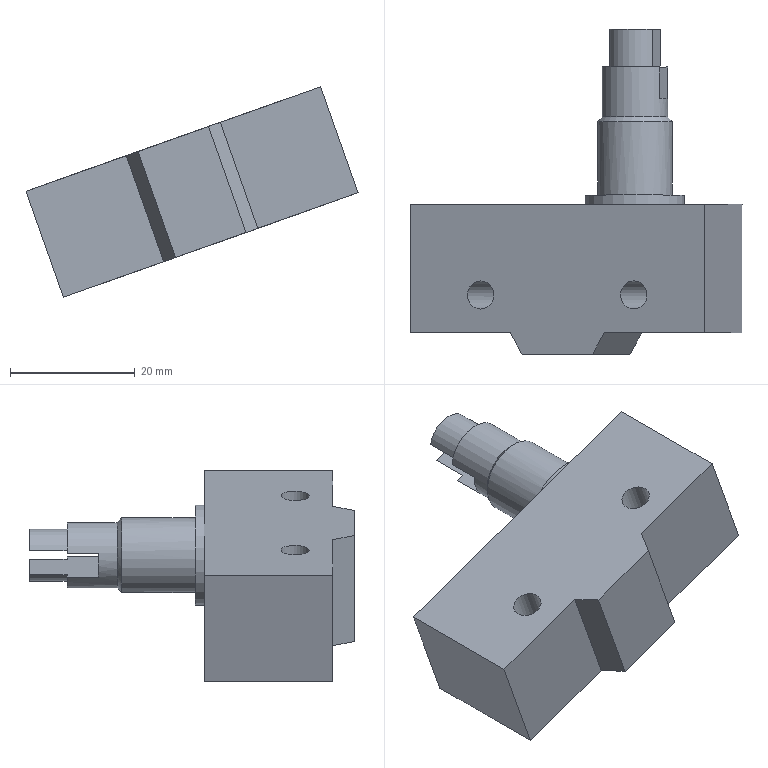Part | STEP file | ELECTRICAL-MICRO-SWITCH3_id10_x_t | 1 solid | 26 faces | box 53.141 x 52 x 33.658 mm | volume 21085 mm3 | plane 18 | cylinder 7 | cone 1 | commonest cylinder face diameters 4.5 x2 8.3 x2 10.5 x1 12 x1 16 x1
STEP:
#1=CARTESIAN_POINT('',(63.608,-176.5,-30.287));
#2=VERTEX_POINT('',#1);
#3=CARTESIAN_POINT('',(56.753,-176.5,-32.715));
#4=VERTEX_POINT('',#3);
#5=CARTESIAN_POINT('',(60.848,-176.5,-33.386));
#6=DIRECTION('',(0.,-1.,0.));
#7=DIRECTION('',(-0.9426,0.,-0.3338));
#8=AXIS2_PLACEMENT_3D('',#5,#6,#7);
#9=CIRCLE('',#8,4.15);
#10=EDGE_CURVE('',#2,#4,#9,.T.);
#11=ORIENTED_EDGE('',*,*,#10,.F.);
#12=CARTESIAN_POINT('',(63.608,-176.5,-30.287));
#13=DIRECTION('',(-0.9426,0.,-0.3338));
#14=VECTOR('',#13,1.);
#15=LINE('',#12,#14);
#16=EDGE_CURVE('',#2,#4,#15,.T.);
#17=ORIENTED_EDGE('',*,*,#16,.T.);
#18=EDGE_LOOP('',(#11,#17));
#19=FACE_OUTER_BOUND('',#18,.T.);
#20=CARTESIAN_POINT('',(60.848,-176.5,-33.386));
#21=DIRECTION('',(0.,1.,0.));
#22=DIRECTION('',(-0.9426,0.,-0.3338));
#23=AXIS2_PLACEMENT_3D('',#20,#21,#22);
#24=PLANE('',#23);
#25=ADVANCED_FACE('',(#19),#24,.T.);
#26=CARTESIAN_POINT('',(56.753,-182.5,-32.715));
#27=VERTEX_POINT('',#26);
#28=CARTESIAN_POINT('',(56.753,-176.5,-32.715));
#29=DIRECTION('',(0.,-1.,0.));
#30=VECTOR('',#29,1.);
#31=LINE('',#28,#30);
#32=EDGE_CURVE('',#4,#27,#31,.T.);
#33=ORIENTED_EDGE('',*,*,#32,.T.);
#34=CARTESIAN_POINT('',(63.608,-182.5,-30.287));
#35=VERTEX_POINT('',#34);
#36=CARTESIAN_POINT('',(60.848,-182.5,-33.386));
#37=DIRECTION('',(0.,-1.,0.));
#38=DIRECTION('',(-0.9426,0.,-0.3338));
#39=AXIS2_PLACEMENT_3D('',#36,#37,#38);
#40=CIRCLE('',#39,4.15);
#41=EDGE_CURVE('',#35,#27,#40,.T.);
#42=ORIENTED_EDGE('',*,*,#41,.F.);
#43=CARTESIAN_POINT('',(63.608,-182.5,-30.287));
#44=DIRECTION('',(0.,1.,0.));
#45=VECTOR('',#44,1.);
#46=LINE('',#43,#45);
#47=EDGE_CURVE('',#35,#2,#46,.T.);
#48=ORIENTED_EDGE('',*,*,#47,.T.);
#49=ORIENTED_EDGE('',*,*,#10,.T.);
#50=EDGE_LOOP('',(#33,#42,#48,#49));
#51=FACE_OUTER_BOUND('',#50,.T.);
#52=CARTESIAN_POINT('',(60.848,-204.325,-33.386));
#53=DIRECTION('',(0.,1.,0.));
#54=DIRECTION('',(-0.9426,0.,-0.3338));
#55=AXIS2_PLACEMENT_3D('',#52,#53,#54);
#56=CYLINDRICAL_SURFACE('',#55,4.15);
#57=ADVANCED_FACE('',(#51),#56,.T.);
#58=CARTESIAN_POINT('',(58.088,-176.5,-36.485));
#59=VERTEX_POINT('',#58);
#60=CARTESIAN_POINT('',(64.943,-176.5,-34.057));
#61=VERTEX_POINT('',#60);
#62=CARTESIAN_POINT('',(60.848,-176.5,-33.386));
#63=DIRECTION('',(0.,-1.,0.));
#64=DIRECTION('',(-0.9426,0.,-0.3338));
#65=AXIS2_PLACEMENT_3D('',#62,#63,#64);
#66=CIRCLE('',#65,4.15);
#67=EDGE_CURVE('',#59,#61,#66,.T.);
#68=ORIENTED_EDGE('',*,*,#67,.F.);
#69=CARTESIAN_POINT('',(58.088,-176.5,-36.485));
#70=DIRECTION('',(0.9426,0.,0.3338));
#71=VECTOR('',#70,1.);
#72=LINE('',#69,#71);
#73=EDGE_CURVE('',#59,#61,#72,.T.);
#74=ORIENTED_EDGE('',*,*,#73,.T.);
#75=EDGE_LOOP('',(#68,#74));
#76=FACE_OUTER_BOUND('',#75,.T.);
#77=CARTESIAN_POINT('',(60.848,-176.5,-33.386));
#78=DIRECTION('',(0.,1.,0.));
#79=DIRECTION('',(-0.9426,0.,-0.3338));
#80=AXIS2_PLACEMENT_3D('',#77,#78,#79);
#81=PLANE('',#80);
#82=ADVANCED_FACE('',(#76),#81,.T.);
#83=CARTESIAN_POINT('',(58.088,-182.5,-36.485));
#84=VERTEX_POINT('',#83);
#85=CARTESIAN_POINT('',(58.088,-182.5,-36.485));
#86=DIRECTION('',(0.,1.,0.));
#87=VECTOR('',#86,1.);
#88=LINE('',#85,#87);
#89=EDGE_CURVE('',#84,#59,#88,.T.);
#90=ORIENTED_EDGE('',*,*,#89,.T.);
#91=ORIENTED_EDGE('',*,*,#67,.T.);
#92=CARTESIAN_POINT('',(64.943,-182.5,-34.057));
#93=VERTEX_POINT('',#92);
#94=CARTESIAN_POINT('',(64.943,-176.5,-34.057));
#95=DIRECTION('',(0.,-1.,0.));
#96=VECTOR('',#95,1.);
#97=LINE('',#94,#96);
#98=EDGE_CURVE('',#61,#93,#97,.T.);
#99=ORIENTED_EDGE('',*,*,#98,.T.);
#100=CARTESIAN_POINT('',(60.848,-182.5,-33.386));
#101=DIRECTION('',(0.,-1.,0.));
#102=DIRECTION('',(-0.9426,0.,-0.3338));
#103=AXIS2_PLACEMENT_3D('',#100,#101,#102);
#104=CIRCLE('',#103,4.15);
#105=EDGE_CURVE('',#84,#93,#104,.T.);
#106=ORIENTED_EDGE('',*,*,#105,.F.);
#107=EDGE_LOOP('',(#90,#91,#99,#106));
#108=FACE_OUTER_BOUND('',#107,.T.);
#109=CARTESIAN_POINT('',(60.848,-204.325,-33.386));
#110=DIRECTION('',(0.,1.,0.));
#111=DIRECTION('',(-0.9426,0.,-0.3338));
#112=AXIS2_PLACEMENT_3D('',#109,#110,#111);
#113=CYLINDRICAL_SURFACE('',#112,4.15);
#114=ADVANCED_FACE('',(#108),#113,.T.);
#115=CARTESIAN_POINT('',(55.605,-187.5,-33.121));
#116=VERTEX_POINT('',#115);
#117=CARTESIAN_POINT('',(56.94,-187.5,-36.892));
#118=VERTEX_POINT('',#117);
#119=CARTESIAN_POINT('',(60.848,-187.5,-33.386));
#120=DIRECTION('',(0.,-1.,0.));
#121=DIRECTION('',(-0.9426,0.,-0.3338));
#122=AXIS2_PLACEMENT_3D('',#119,#120,#121);
#123=CIRCLE('',#122,5.25);
#124=EDGE_CURVE('',#116,#118,#123,.T.);
#125=ORIENTED_EDGE('',*,*,#124,.F.);
#126=CARTESIAN_POINT('',(64.756,-187.5,-29.88));
#127=VERTEX_POINT('',#126);
#128=CARTESIAN_POINT('',(55.605,-187.5,-33.121));
#129=DIRECTION('',(0.9426,0.,0.3338));
#130=VECTOR('',#129,1.);
#131=LINE('',#128,#130);
#132=EDGE_CURVE('',#116,#127,#131,.T.);
#133=ORIENTED_EDGE('',*,*,#132,.T.);
#134=CARTESIAN_POINT('',(66.091,-187.5,-33.651));
#135=VERTEX_POINT('',#134);
#136=CARTESIAN_POINT('',(60.848,-187.5,-33.386));
#137=DIRECTION('',(0.,-1.,0.));
#138=DIRECTION('',(-0.9426,0.,-0.3338));
#139=AXIS2_PLACEMENT_3D('',#136,#137,#138);
#140=CIRCLE('',#139,5.25);
#141=EDGE_CURVE('',#135,#127,#140,.T.);
#142=ORIENTED_EDGE('',*,*,#141,.F.);
#143=CARTESIAN_POINT('',(66.091,-187.5,-33.651));
#144=DIRECTION('',(-0.9426,0.,-0.3338));
#145=VECTOR('',#144,1.);
#146=LINE('',#143,#145);
#147=EDGE_CURVE('',#135,#118,#146,.T.);
#148=ORIENTED_EDGE('',*,*,#147,.T.);
#149=EDGE_LOOP('',(#125,#133,#142,#148));
#150=FACE_OUTER_BOUND('',#149,.T.);
#151=CARTESIAN_POINT('',(74.32,-187.5,-26.494));
#152=DIRECTION('',(0.,-1.,0.));
#153=DIRECTION('',(0.9426,0.,0.3338));
#154=AXIS2_PLACEMENT_3D('',#151,#152,#153);
#155=PLANE('',#154);
#156=ADVANCED_FACE('',(#150),#155,.F.);
#157=CARTESIAN_POINT('',(64.756,-182.5,-29.88));
#158=VERTEX_POINT('',#157);
#159=CARTESIAN_POINT('',(60.18,-182.5,-31.501));
#160=DIRECTION('',(-0.9426,0.,-0.3338));
#161=VECTOR('',#160,1.);
#162=LINE('',#159,#161);
#163=EDGE_CURVE('',#158,#35,#162,.T.);
#164=ORIENTED_EDGE('',*,*,#163,.F.);
#165=CARTESIAN_POINT('',(64.756,-204.325,-29.88));
#166=DIRECTION('',(0.,1.,0.));
#167=VECTOR('',#166,1.);
#168=LINE('',#165,#167);
#169=EDGE_CURVE('',#127,#158,#168,.T.);
#170=ORIENTED_EDGE('',*,*,#169,.F.);
#171=ORIENTED_EDGE('',*,*,#132,.F.);
#172=CARTESIAN_POINT('',(55.605,-182.5,-33.121));
#173=VERTEX_POINT('',#172);
#174=CARTESIAN_POINT('',(55.605,-204.325,-33.121));
#175=DIRECTION('',(0.,-1.,0.));
#176=VECTOR('',#175,1.);
#177=LINE('',#174,#176);
#178=EDGE_CURVE('',#173,#116,#177,.T.);
#179=ORIENTED_EDGE('',*,*,#178,.F.);
#180=CARTESIAN_POINT('',(60.18,-182.5,-31.501));
#181=DIRECTION('',(-0.9426,0.,-0.3338));
#182=VECTOR('',#181,1.);
#183=LINE('',#180,#182);
#184=EDGE_CURVE('',#27,#173,#183,.T.);
#185=ORIENTED_EDGE('',*,*,#184,.F.);
#186=ORIENTED_EDGE('',*,*,#32,.F.);
#187=ORIENTED_EDGE('',*,*,#16,.F.);
#188=ORIENTED_EDGE('',*,*,#47,.F.);
#189=EDGE_LOOP('',(#164,#170,#171,#179,#185,#186,#187,#188));
#190=FACE_OUTER_BOUND('',#189,.T.);
#191=CARTESIAN_POINT('',(74.32,-176.5,-26.494));
#192=DIRECTION('',(-0.3338,0.,0.9426));
#193=DIRECTION('',(0.8886,0.3338,0.3147));
#194=AXIS2_PLACEMENT_3D('',#191,#192,#193);
#195=PLANE('',#194);
#196=ADVANCED_FACE('',(#190),#195,.F.);
#197=CARTESIAN_POINT('',(60.848,-182.5,-33.386));
#198=DIRECTION('',(0.,-1.,0.));
#199=DIRECTION('',(-0.9426,0.,-0.3338));
#200=AXIS2_PLACEMENT_3D('',#197,#198,#199);
#201=CIRCLE('',#200,5.25);
#202=EDGE_CURVE('',#158,#173,#201,.T.);
#203=ORIENTED_EDGE('',*,*,#202,.F.);
#204=ORIENTED_EDGE('',*,*,#163,.T.);
#205=ORIENTED_EDGE('',*,*,#41,.T.);
#206=ORIENTED_EDGE('',*,*,#184,.T.);
#207=EDGE_LOOP('',(#203,#204,#205,#206));
#208=FACE_OUTER_BOUND('',#207,.T.);
#209=CARTESIAN_POINT('',(60.848,-182.5,-33.386));
#210=DIRECTION('',(0.,1.,0.));
#211=DIRECTION('',(-0.9426,0.,-0.3338));
#212=AXIS2_PLACEMENT_3D('',#209,#210,#211);
#213=PLANE('',#212);
#214=ADVANCED_FACE('',(#208),#213,.T.);
#215=ORIENTED_EDGE('',*,*,#105,.T.);
#216=CARTESIAN_POINT('',(66.091,-182.5,-33.651));
#217=VERTEX_POINT('',#216);
#218=CARTESIAN_POINT('',(64.943,-182.5,-34.057));
#219=DIRECTION('',(0.9426,0.,0.3338));
#220=VECTOR('',#219,1.);
#221=LINE('',#218,#220);
#222=EDGE_CURVE('',#93,#217,#221,.T.);
#223=ORIENTED_EDGE('',*,*,#222,.T.);
#224=CARTESIAN_POINT('',(56.94,-182.5,-36.892));
#225=VERTEX_POINT('',#224);
#226=CARTESIAN_POINT('',(60.848,-182.5,-33.386));
#227=DIRECTION('',(0.,-1.,0.));
#228=DIRECTION('',(-0.9426,0.,-0.3338));
#229=AXIS2_PLACEMENT_3D('',#226,#227,#228);
#230=CIRCLE('',#229,5.25);
#231=EDGE_CURVE('',#225,#217,#230,.T.);
#232=ORIENTED_EDGE('',*,*,#231,.F.);
#233=CARTESIAN_POINT('',(56.94,-182.5,-36.892));
#234=DIRECTION('',(0.9426,0.,0.3338));
#235=VECTOR('',#234,1.);
#236=LINE('',#233,#235);
#237=EDGE_CURVE('',#225,#84,#236,.T.);
#238=ORIENTED_EDGE('',*,*,#237,.T.);
#239=EDGE_LOOP('',(#215,#223,#232,#238));
#240=FACE_OUTER_BOUND('',#239,.T.);
#241=CARTESIAN_POINT('',(60.848,-182.5,-33.386));
#242=DIRECTION('',(0.,1.,0.));
#243=DIRECTION('',(-0.9426,0.,-0.3338));
#244=AXIS2_PLACEMENT_3D('',#241,#242,#243);
#245=PLANE('',#244);
#246=ADVANCED_FACE('',(#240),#245,.T.);
#247=ORIENTED_EDGE('',*,*,#237,.F.);
#248=CARTESIAN_POINT('',(56.94,-204.325,-36.892));
#249=DIRECTION('',(0.,1.,0.));
#250=VECTOR('',#249,1.);
#251=LINE('',#248,#250);
#252=EDGE_CURVE('',#118,#225,#251,.T.);
#253=ORIENTED_EDGE('',*,*,#252,.F.);
#254=ORIENTED_EDGE('',*,*,#147,.F.);
#255=CARTESIAN_POINT('',(66.091,-204.325,-33.651));
#256=DIRECTION('',(0.,-1.,0.));
#257=VECTOR('',#256,1.);
#258=LINE('',#255,#257);
#259=EDGE_CURVE('',#217,#135,#258,.T.);
#260=ORIENTED_EDGE('',*,*,#259,.F.);
#261=ORIENTED_EDGE('',*,*,#222,.F.);
#262=ORIENTED_EDGE('',*,*,#98,.F.);
#263=ORIENTED_EDGE('',*,*,#73,.F.);
#264=ORIENTED_EDGE('',*,*,#89,.F.);
#265=EDGE_LOOP('',(#247,#253,#254,#260,#261,#262,#263,#264));
#266=FACE_OUTER_BOUND('',#265,.T.);
#267=CARTESIAN_POINT('',(75.655,-187.5,-30.264));
#268=DIRECTION('',(0.3338,0.,-0.9426));
#269=DIRECTION('',(-0.8886,-0.3338,-0.3147));
#270=AXIS2_PLACEMENT_3D('',#267,#268,#269);
#271=PLANE('',#270);
#272=ADVANCED_FACE('',(#266),#271,.F.);
#273=CARTESIAN_POINT('',(59.095,-190.5,-28.437));
#274=VERTEX_POINT('',#273);
#275=CARTESIAN_POINT('',(60.848,-190.5,-33.386));
#276=DIRECTION('',(0.,-1.,0.));
#277=DIRECTION('',(-0.3338,0.,0.9426));
#278=AXIS2_PLACEMENT_3D('',#275,#276,#277);
#279=CIRCLE('',#278,5.25);
#280=EDGE_CURVE('',#274,#274,#279,.T.);
#281=ORIENTED_EDGE('',*,*,#280,.F.);
#282=EDGE_LOOP('',(#281));
#283=FACE_BOUND('',#282,.T.);
#284=ORIENTED_EDGE('',*,*,#231,.T.);
#285=ORIENTED_EDGE('',*,*,#259,.T.);
#286=ORIENTED_EDGE('',*,*,#141,.T.);
#287=ORIENTED_EDGE('',*,*,#169,.T.);
#288=ORIENTED_EDGE('',*,*,#202,.T.);
#289=ORIENTED_EDGE('',*,*,#178,.T.);
#290=ORIENTED_EDGE('',*,*,#124,.T.);
#291=ORIENTED_EDGE('',*,*,#252,.T.);
#292=EDGE_LOOP('',(#284,#285,#286,#287,#288,#289,#290,#291));
#293=FACE_BOUND('',#292,.T.);
#294=CARTESIAN_POINT('',(60.848,-204.325,-33.386));
#295=DIRECTION('',(0.,1.,0.));
#296=DIRECTION('',(-0.9426,0.,-0.3338));
#297=AXIS2_PLACEMENT_3D('',#294,#295,#296);
#298=CYLINDRICAL_SURFACE('',#297,5.25);
#299=ADVANCED_FACE('',(#283,#293),#298,.T.);
#300=ORIENTED_EDGE('',*,*,#280,.T.);
#301=EDGE_LOOP('',(#300));
#302=FACE_BOUND('',#301,.T.);
#303=CARTESIAN_POINT('',(55.192,-191.25,-35.389));
#304=VERTEX_POINT('',#303);
#305=CARTESIAN_POINT('',(60.848,-191.25,-33.386));
#306=DIRECTION('',(0.,-1.,0.));
#307=DIRECTION('',(-0.9426,0.,-0.3338));
#308=AXIS2_PLACEMENT_3D('',#305,#306,#307);
#309=CIRCLE('',#308,6.);
#310=EDGE_CURVE('',#304,#304,#309,.T.);
#311=ORIENTED_EDGE('',*,*,#310,.F.);
#312=EDGE_LOOP('',(#311));
#313=FACE_BOUND('',#312,.T.);
#314=CARTESIAN_POINT('',(60.848,-191.25,-33.386));
#315=DIRECTION('',(0.,-1.,0.));
#316=DIRECTION('',(0.9426,0.,0.3338));
#317=AXIS2_PLACEMENT_3D('',#314,#315,#316);
#318=CONICAL_SURFACE('',#317,6.,45.);
#319=ADVANCED_FACE('',(#302,#313),#318,.T.);
#320=ORIENTED_EDGE('',*,*,#310,.T.);
#321=EDGE_LOOP('',(#320));
#322=FACE_BOUND('',#321,.T.);
#323=CARTESIAN_POINT('',(55.192,-203.,-35.389));
#324=VERTEX_POINT('',#323);
#325=CARTESIAN_POINT('',(60.848,-203.,-33.386));
#326=DIRECTION('',(0.,-1.,0.));
#327=DIRECTION('',(-0.9426,0.,-0.3338));
#328=AXIS2_PLACEMENT_3D('',#325,#326,#327);
#329=CIRCLE('',#328,6.);
#330=EDGE_CURVE('',#324,#324,#329,.T.);
#331=ORIENTED_EDGE('',*,*,#330,.F.);
#332=EDGE_LOOP('',(#331));
#333=FACE_BOUND('',#332,.T.);
#334=CARTESIAN_POINT('',(60.848,-204.325,-33.386));
#335=DIRECTION('',(0.,1.,0.));
#336=DIRECTION('',(-0.9426,0.,-0.3338));
#337=AXIS2_PLACEMENT_3D('',#334,#335,#336);
#338=CYLINDRICAL_SURFACE('',#337,6.);
#339=ADVANCED_FACE('',(#322,#333),#338,.T.);
#340=ORIENTED_EDGE('',*,*,#330,.T.);
#341=EDGE_LOOP('',(#340));
#342=FACE_BOUND('',#341,.T.);
#343=CARTESIAN_POINT('',(53.307,-203.,-36.056));
#344=VERTEX_POINT('',#343);
#345=CARTESIAN_POINT('',(60.848,-203.,-33.386));
#346=DIRECTION('',(0.,-1.,0.));
#347=DIRECTION('',(-0.9426,0.,-0.3338));
#348=AXIS2_PLACEMENT_3D('',#345,#346,#347);
#349=CIRCLE('',#348,8.);
#350=EDGE_CURVE('',#344,#344,#349,.T.);
#351=ORIENTED_EDGE('',*,*,#350,.F.);
#352=EDGE_LOOP('',(#351));
#353=FACE_BOUND('',#352,.T.);
#354=CARTESIAN_POINT('',(-35.179,-203.,-57.843));
#355=DIRECTION('',(0.,1.,0.));
#356=DIRECTION('',(-0.9426,0.,-0.3338));
#357=AXIS2_PLACEMENT_3D('',#354,#355,#356);
#358=PLANE('',#357);
#359=ADVANCED_FACE('',(#342,#353),#358,.T.);
#360=ORIENTED_EDGE('',*,*,#350,.T.);
#361=EDGE_LOOP('',(#360));
#362=FACE_BOUND('',#361,.T.);
#363=CARTESIAN_POINT('',(53.307,-204.5,-36.056));
#364=VERTEX_POINT('',#363);
#365=CARTESIAN_POINT('',(60.848,-204.5,-33.386));
#366=DIRECTION('',(0.,-1.,0.));
#367=DIRECTION('',(-0.9426,0.,-0.3338));
#368=AXIS2_PLACEMENT_3D('',#365,#366,#367);
#369=CIRCLE('',#368,8.);
#370=EDGE_CURVE('',#364,#364,#369,.T.);
#371=ORIENTED_EDGE('',*,*,#370,.F.);
#372=EDGE_LOOP('',(#371));
#373=FACE_BOUND('',#372,.T.);
#374=CARTESIAN_POINT('',(60.848,-204.5,-33.386));
#375=DIRECTION('',(0.,1.,0.));
#376=DIRECTION('',(-0.9426,0.,-0.3338));
#377=AXIS2_PLACEMENT_3D('',#374,#375,#376);
#378=CYLINDRICAL_SURFACE('',#377,8.);
#379=ADVANCED_FACE('',(#362,#373),#378,.T.);
#380=CARTESIAN_POINT('',(62.671,-218.249,-23.193));
#381=VERTEX_POINT('',#380);
#382=CARTESIAN_POINT('',(60.672,-219.,-23.901));
#383=DIRECTION('',(0.3338,0.,-0.9426));
#384=DIRECTION('',(0.8886,0.3338,0.3147));
#385=AXIS2_PLACEMENT_3D('',#382,#383,#384);
#386=CIRCLE('',#385,2.25);
#387=EDGE_CURVE('',#381,#381,#386,.T.);
#388=ORIENTED_EDGE('',*,*,#387,.T.);
#389=EDGE_LOOP('',(#388));
#390=FACE_BOUND('',#389,.T.);
#391=CARTESIAN_POINT('',(38.162,-218.249,-31.872));
#392=VERTEX_POINT('',#391);
#393=CARTESIAN_POINT('',(36.163,-219.,-32.58));
#394=DIRECTION('',(0.3338,0.,-0.9426));
#395=DIRECTION('',(0.8886,0.3338,0.3147));
#396=AXIS2_PLACEMENT_3D('',#393,#394,#395);
#397=CIRCLE('',#396,2.25);
#398=EDGE_CURVE('',#392,#392,#397,.T.);
#399=ORIENTED_EDGE('',*,*,#398,.T.);
#400=EDGE_LOOP('',(#399));
#401=FACE_BOUND('',#400,.T.);
#402=CARTESIAN_POINT('',(24.851,-225.,-36.585));
#403=VERTEX_POINT('',#402);
#404=CARTESIAN_POINT('',(24.851,-204.5,-36.585));
#405=VERTEX_POINT('',#404);
#406=CARTESIAN_POINT('',(24.851,-204.5,-36.585));
#407=DIRECTION('',(0.,1.,0.));
#408=VECTOR('',#407,1.);
#409=LINE('',#406,#408);
#410=EDGE_CURVE('',#403,#405,#409,.T.);
#411=ORIENTED_EDGE('',*,*,#410,.F.);
#412=CARTESIAN_POINT('',(40.876,-225.,-30.911));
#413=VERTEX_POINT('',#412);
#414=CARTESIAN_POINT('',(24.851,-225.,-36.585));
#415=DIRECTION('',(-0.9426,0.,-0.3338));
#416=VECTOR('',#415,1.);
#417=LINE('',#414,#416);
#418=EDGE_CURVE('',#413,#403,#417,.T.);
#419=ORIENTED_EDGE('',*,*,#418,.F.);
#420=CARTESIAN_POINT('',(42.781,-228.5,-30.236));
#421=VERTEX_POINT('',#420);
#422=CARTESIAN_POINT('',(40.876,-225.,-30.911));
#423=DIRECTION('',(-0.4713,0.866,-0.1669));
#424=VECTOR('',#423,1.);
#425=LINE('',#422,#424);
#426=EDGE_CURVE('',#421,#413,#425,.T.);
#427=ORIENTED_EDGE('',*,*,#426,.F.);
#428=CARTESIAN_POINT('',(54.054,-228.5,-26.244));
#429=VERTEX_POINT('',#428);
#430=CARTESIAN_POINT('',(42.781,-228.5,-30.236));
#431=DIRECTION('',(-0.9426,0.,-0.3338));
#432=VECTOR('',#431,1.);
#433=LINE('',#430,#432);
#434=EDGE_CURVE('',#429,#421,#433,.T.);
#435=ORIENTED_EDGE('',*,*,#434,.F.);
#436=CARTESIAN_POINT('',(55.958,-225.,-25.57));
#437=VERTEX_POINT('',#436);
#438=CARTESIAN_POINT('',(54.054,-228.5,-26.244));
#439=DIRECTION('',(-0.4713,-0.866,-0.1669));
#440=VECTOR('',#439,1.);
#441=LINE('',#438,#440);
#442=EDGE_CURVE('',#437,#429,#441,.T.);
#443=ORIENTED_EDGE('',*,*,#442,.F.);
#444=CARTESIAN_POINT('',(71.983,-225.,-19.895));
#445=VERTEX_POINT('',#444);
#446=CARTESIAN_POINT('',(55.958,-225.,-25.57));
#447=DIRECTION('',(-0.9426,0.,-0.3338));
#448=VECTOR('',#447,1.);
#449=LINE('',#446,#448);
#450=EDGE_CURVE('',#445,#437,#449,.T.);
#451=ORIENTED_EDGE('',*,*,#450,.F.);
#452=CARTESIAN_POINT('',(71.983,-204.5,-19.895));
#453=VERTEX_POINT('',#452);
#454=CARTESIAN_POINT('',(71.983,-225.,-19.895));
#455=DIRECTION('',(0.,-1.,0.));
#456=VECTOR('',#455,1.);
#457=LINE('',#454,#456);
#458=EDGE_CURVE('',#453,#445,#457,.T.);
#459=ORIENTED_EDGE('',*,*,#458,.F.);
#460=CARTESIAN_POINT('',(71.983,-204.5,-19.895));
#461=DIRECTION('',(0.9426,0.,0.3338));
#462=VECTOR('',#461,1.);
#463=LINE('',#460,#462);
#464=EDGE_CURVE('',#405,#453,#463,.T.);
#465=ORIENTED_EDGE('',*,*,#464,.F.);
#466=EDGE_LOOP('',(#411,#419,#427,#435,#443,#451,#459,#465));
#467=FACE_BOUND('',#466,.T.);
#468=CARTESIAN_POINT('',(-35.179,-361.039,-57.843));
#469=DIRECTION('',(-0.3338,0.,0.9426));
#470=DIRECTION('',(0.8886,0.3338,0.3147));
#471=AXIS2_PLACEMENT_3D('',#468,#469,#470);
#472=PLANE('',#471);
#473=ADVANCED_FACE('',(#390,#401,#467),#472,.T.);
#474=CARTESIAN_POINT('',(30.86,-225.,-53.553));
#475=VERTEX_POINT('',#474);
#476=CARTESIAN_POINT('',(30.86,-225.,-53.553));
#477=DIRECTION('',(-0.3338,0.,0.9426));
#478=VECTOR('',#477,1.);
#479=LINE('',#476,#478);
#480=EDGE_CURVE('',#475,#403,#479,.T.);
#481=ORIENTED_EDGE('',*,*,#480,.F.);
#482=CARTESIAN_POINT('',(46.885,-225.,-47.878));
#483=VERTEX_POINT('',#482);
#484=CARTESIAN_POINT('',(30.86,-225.,-53.553));
#485=DIRECTION('',(0.9426,0.,0.3338));
#486=VECTOR('',#485,1.);
#487=LINE('',#484,#486);
#488=EDGE_CURVE('',#475,#483,#487,.T.);
#489=ORIENTED_EDGE('',*,*,#488,.T.);
#490=CARTESIAN_POINT('',(46.885,-225.,-47.878));
#491=DIRECTION('',(0.3338,0.,-0.9426));
#492=VECTOR('',#491,1.);
#493=LINE('',#490,#492);
#494=EDGE_CURVE('',#413,#483,#493,.T.);
#495=ORIENTED_EDGE('',*,*,#494,.F.);
#496=ORIENTED_EDGE('',*,*,#418,.T.);
#497=EDGE_LOOP('',(#481,#489,#495,#496));
#498=FACE_OUTER_BOUND('',#497,.T.);
#499=CARTESIAN_POINT('',(30.86,-225.,-53.553));
#500=DIRECTION('',(0.,-1.,0.));
#501=DIRECTION('',(0.9426,0.,0.3338));
#502=AXIS2_PLACEMENT_3D('',#499,#500,#501);
#503=PLANE('',#502);
#504=ADVANCED_FACE('',(#498),#503,.T.);
#505=ORIENTED_EDGE('',*,*,#494,.T.);
#506=CARTESIAN_POINT('',(48.789,-228.5,-47.204));
#507=VERTEX_POINT('',#506);
#508=CARTESIAN_POINT('',(46.885,-225.,-47.878));
#509=DIRECTION('',(0.4713,-0.866,0.1669));
#510=VECTOR('',#509,1.);
#511=LINE('',#508,#510);
#512=EDGE_CURVE('',#483,#507,#511,.T.);
#513=ORIENTED_EDGE('',*,*,#512,.T.);
#514=CARTESIAN_POINT('',(48.789,-228.5,-47.204));
#515=DIRECTION('',(0.3338,0.,-0.9426));
#516=VECTOR('',#515,1.);
#517=LINE('',#514,#516);
#518=EDGE_CURVE('',#421,#507,#517,.T.);
#519=ORIENTED_EDGE('',*,*,#518,.F.);
#520=ORIENTED_EDGE('',*,*,#426,.T.);
#521=EDGE_LOOP('',(#505,#513,#519,#520));
#522=FACE_OUTER_BOUND('',#521,.T.);
#523=CARTESIAN_POINT('',(46.885,-225.,-47.878));
#524=DIRECTION('',(-0.8164,-0.5,-0.2891));
#525=DIRECTION('',(0.4713,-0.866,0.1669));
#526=AXIS2_PLACEMENT_3D('',#523,#524,#525);
#527=PLANE('',#526);
#528=ADVANCED_FACE('',(#522),#527,.T.);
#529=ORIENTED_EDGE('',*,*,#518,.T.);
#530=CARTESIAN_POINT('',(60.062,-228.5,-43.212));
#531=VERTEX_POINT('',#530);
#532=CARTESIAN_POINT('',(48.789,-228.5,-47.204));
#533=DIRECTION('',(0.9426,0.,0.3338));
#534=VECTOR('',#533,1.);
#535=LINE('',#532,#534);
#536=EDGE_CURVE('',#507,#531,#535,.T.);
#537=ORIENTED_EDGE('',*,*,#536,.T.);
#538=CARTESIAN_POINT('',(60.062,-228.5,-43.212));
#539=DIRECTION('',(0.3338,0.,-0.9426));
#540=VECTOR('',#539,1.);
#541=LINE('',#538,#540);
#542=EDGE_CURVE('',#429,#531,#541,.T.);
#543=ORIENTED_EDGE('',*,*,#542,.F.);
#544=ORIENTED_EDGE('',*,*,#434,.T.);
#545=EDGE_LOOP('',(#529,#537,#543,#544));
#546=FACE_OUTER_BOUND('',#545,.T.);
#547=CARTESIAN_POINT('',(48.789,-228.5,-47.204));
#548=DIRECTION('',(0.,-1.,0.));
#549=DIRECTION('',(0.9426,0.,0.3338));
#550=AXIS2_PLACEMENT_3D('',#547,#548,#549);
#551=PLANE('',#550);
#552=ADVANCED_FACE('',(#546),#551,.T.);
#553=ORIENTED_EDGE('',*,*,#542,.T.);
#554=CARTESIAN_POINT('',(61.967,-225.,-42.537));
#555=VERTEX_POINT('',#554);
#556=CARTESIAN_POINT('',(60.062,-228.5,-43.212));
#557=DIRECTION('',(0.4713,0.866,0.1669));
#558=VECTOR('',#557,1.);
#559=LINE('',#556,#558);
#560=EDGE_CURVE('',#531,#555,#559,.T.);
#561=ORIENTED_EDGE('',*,*,#560,.T.);
#562=CARTESIAN_POINT('',(61.967,-225.,-42.537));
#563=DIRECTION('',(0.3338,0.,-0.9426));
#564=VECTOR('',#563,1.);
#565=LINE('',#562,#564);
#566=EDGE_CURVE('',#437,#555,#565,.T.);
#567=ORIENTED_EDGE('',*,*,#566,.F.);
#568=ORIENTED_EDGE('',*,*,#442,.T.);
#569=EDGE_LOOP('',(#553,#561,#567,#568));
#570=FACE_OUTER_BOUND('',#569,.T.);
#571=CARTESIAN_POINT('',(60.062,-228.5,-43.212));
#572=DIRECTION('',(0.8164,-0.5,0.2891));
#573=DIRECTION('',(0.4713,0.866,0.1669));
#574=AXIS2_PLACEMENT_3D('',#571,#572,#573);
#575=PLANE('',#574);
#576=ADVANCED_FACE('',(#570),#575,.T.);
#577=ORIENTED_EDGE('',*,*,#566,.T.);
#578=CARTESIAN_POINT('',(77.992,-225.,-36.863));
#579=VERTEX_POINT('',#578);
#580=CARTESIAN_POINT('',(61.967,-225.,-42.537));
#581=DIRECTION('',(0.9426,0.,0.3338));
#582=VECTOR('',#581,1.);
#583=LINE('',#580,#582);
#584=EDGE_CURVE('',#555,#579,#583,.T.);
#585=ORIENTED_EDGE('',*,*,#584,.T.);
#586=CARTESIAN_POINT('',(77.992,-225.,-36.863));
#587=DIRECTION('',(0.3338,0.,-0.9426));
#588=VECTOR('',#587,1.);
#589=LINE('',#586,#588);
#590=EDGE_CURVE('',#445,#579,#589,.T.);
#591=ORIENTED_EDGE('',*,*,#590,.F.);
#592=ORIENTED_EDGE('',*,*,#450,.T.);
#593=EDGE_LOOP('',(#577,#585,#591,#592));
#594=FACE_OUTER_BOUND('',#593,.T.);
#595=CARTESIAN_POINT('',(61.967,-225.,-42.537));
#596=DIRECTION('',(0.,-1.,0.));
#597=DIRECTION('',(0.9426,0.,0.3338));
#598=AXIS2_PLACEMENT_3D('',#595,#596,#597);
#599=PLANE('',#598);
#600=ADVANCED_FACE('',(#594),#599,.T.);
#601=ORIENTED_EDGE('',*,*,#590,.T.);
#602=CARTESIAN_POINT('',(77.992,-204.5,-36.863));
#603=VERTEX_POINT('',#602);
#604=CARTESIAN_POINT('',(77.992,-225.,-36.863));
#605=DIRECTION('',(0.,1.,0.));
#606=VECTOR('',#605,1.);
#607=LINE('',#604,#606);
#608=EDGE_CURVE('',#579,#603,#607,.T.);
#609=ORIENTED_EDGE('',*,*,#608,.T.);
#610=CARTESIAN_POINT('',(77.992,-204.5,-36.863));
#611=DIRECTION('',(0.3338,0.,-0.9426));
#612=VECTOR('',#611,1.);
#613=LINE('',#610,#612);
#614=EDGE_CURVE('',#453,#603,#613,.T.);
#615=ORIENTED_EDGE('',*,*,#614,.F.);
#616=ORIENTED_EDGE('',*,*,#458,.T.);
#617=EDGE_LOOP('',(#601,#609,#615,#616));
#618=FACE_OUTER_BOUND('',#617,.T.);
#619=CARTESIAN_POINT('',(77.992,-225.,-36.863));
#620=DIRECTION('',(0.9426,0.,0.3338));
#621=DIRECTION('',(0.,1.,0.));
#622=AXIS2_PLACEMENT_3D('',#619,#620,#621);
#623=PLANE('',#622);
#624=ADVANCED_FACE('',(#618),#623,.T.);
#625=ORIENTED_EDGE('',*,*,#370,.T.);
#626=EDGE_LOOP('',(#625));
#627=FACE_BOUND('',#626,.T.);
#628=ORIENTED_EDGE('',*,*,#614,.T.);
#629=CARTESIAN_POINT('',(30.86,-204.5,-53.553));
#630=VERTEX_POINT('',#629);
#631=CARTESIAN_POINT('',(77.992,-204.5,-36.863));
#632=DIRECTION('',(-0.9426,0.,-0.3338));
#633=VECTOR('',#632,1.);
#634=LINE('',#631,#633);
#635=EDGE_CURVE('',#603,#630,#634,.T.);
#636=ORIENTED_EDGE('',*,*,#635,.T.);
#637=CARTESIAN_POINT('',(30.86,-204.5,-53.553));
#638=DIRECTION('',(0.3338,0.,-0.9426));
#639=VECTOR('',#638,1.);
#640=LINE('',#637,#639);
#641=EDGE_CURVE('',#405,#630,#640,.T.);
#642=ORIENTED_EDGE('',*,*,#641,.F.);
#643=ORIENTED_EDGE('',*,*,#464,.T.);
#644=EDGE_LOOP('',(#628,#636,#642,#643));
#645=FACE_BOUND('',#644,.T.);
#646=CARTESIAN_POINT('',(77.992,-204.5,-36.863));
#647=DIRECTION('',(0.,1.,0.));
#648=DIRECTION('',(-0.9426,0.,-0.3338));
#649=AXIS2_PLACEMENT_3D('',#646,#647,#648);
#650=PLANE('',#649);
#651=ADVANCED_FACE('',(#627,#645),#650,.T.);
#652=ORIENTED_EDGE('',*,*,#641,.T.);
#653=CARTESIAN_POINT('',(30.86,-204.5,-53.553));
#654=DIRECTION('',(0.,-1.,0.));
#655=VECTOR('',#654,1.);
#656=LINE('',#653,#655);
#657=EDGE_CURVE('',#630,#475,#656,.T.);
#658=ORIENTED_EDGE('',*,*,#657,.T.);
#659=ORIENTED_EDGE('',*,*,#480,.T.);
#660=ORIENTED_EDGE('',*,*,#410,.T.);
#661=EDGE_LOOP('',(#652,#658,#659,#660));
#662=FACE_OUTER_BOUND('',#661,.T.);
#663=CARTESIAN_POINT('',(30.86,-204.5,-53.553));
#664=DIRECTION('',(-0.9426,0.,-0.3338));
#665=DIRECTION('',(0.,-1.,0.));
#666=AXIS2_PLACEMENT_3D('',#663,#664,#665);
#667=PLANE('',#666);
#668=ADVANCED_FACE('',(#662),#667,.T.);
#669=ORIENTED_EDGE('',*,*,#398,.F.);
#670=EDGE_LOOP('',(#669));
#671=FACE_BOUND('',#670,.T.);
#672=CARTESIAN_POINT('',(44.171,-218.249,-48.839));
#673=VERTEX_POINT('',#672);
#674=CARTESIAN_POINT('',(42.171,-219.,-49.547));
#675=DIRECTION('',(0.3338,0.,-0.9426));
#676=DIRECTION('',(0.8886,0.3338,0.3147));
#677=AXIS2_PLACEMENT_3D('',#674,#675,#676);
#678=CIRCLE('',#677,2.25);
#679=EDGE_CURVE('',#673,#673,#678,.T.);
#680=ORIENTED_EDGE('',*,*,#679,.T.);
#681=EDGE_LOOP('',(#680));
#682=FACE_BOUND('',#681,.T.);
#683=CARTESIAN_POINT('',(42.171,-219.,-49.547));
#684=DIRECTION('',(-0.3338,0.,0.9426));
#685=DIRECTION('',(0.8886,0.3338,0.3147));
#686=AXIS2_PLACEMENT_3D('',#683,#684,#685);
#687=CYLINDRICAL_SURFACE('',#686,2.25);
#688=ADVANCED_FACE('',(#671,#682),#687,.F.);
#689=ORIENTED_EDGE('',*,*,#387,.F.);
#690=EDGE_LOOP('',(#689));
#691=FACE_BOUND('',#690,.T.);
#692=CARTESIAN_POINT('',(68.679,-218.249,-40.16));
#693=VERTEX_POINT('',#692);
#694=CARTESIAN_POINT('',(66.68,-219.,-40.868));
#695=DIRECTION('',(0.3338,0.,-0.9426));
#696=DIRECTION('',(0.8886,0.3338,0.3147));
#697=AXIS2_PLACEMENT_3D('',#694,#695,#696);
#698=CIRCLE('',#697,2.25);
#699=EDGE_CURVE('',#693,#693,#698,.T.);
#700=ORIENTED_EDGE('',*,*,#699,.T.);
#701=EDGE_LOOP('',(#700));
#702=FACE_BOUND('',#701,.T.);
#703=CARTESIAN_POINT('',(66.68,-219.,-40.868));
#704=DIRECTION('',(-0.3338,0.,0.9426));
#705=DIRECTION('',(0.8886,0.3338,0.3147));
#706=AXIS2_PLACEMENT_3D('',#703,#704,#705);
#707=CYLINDRICAL_SURFACE('',#706,2.25);
#708=ADVANCED_FACE('',(#691,#702),#707,.F.);
#709=ORIENTED_EDGE('',*,*,#699,.F.);
#710=EDGE_LOOP('',(#709));
#711=FACE_BOUND('',#710,.T.);
#712=ORIENTED_EDGE('',*,*,#679,.F.);
#713=EDGE_LOOP('',(#712));
#714=FACE_BOUND('',#713,.T.);
#715=ORIENTED_EDGE('',*,*,#635,.F.);
#716=ORIENTED_EDGE('',*,*,#608,.F.);
#717=ORIENTED_EDGE('',*,*,#584,.F.);
#718=ORIENTED_EDGE('',*,*,#560,.F.);
#719=ORIENTED_EDGE('',*,*,#536,.F.);
#720=ORIENTED_EDGE('',*,*,#512,.F.);
#721=ORIENTED_EDGE('',*,*,#488,.F.);
#722=ORIENTED_EDGE('',*,*,#657,.F.);
#723=EDGE_LOOP('',(#715,#716,#717,#718,#719,#720,#721,#722));
#724=FACE_BOUND('',#723,.T.);
#725=CARTESIAN_POINT('',(-29.17,-361.039,-74.811));
#726=DIRECTION('',(-0.3338,0.,0.9426));
#727=DIRECTION('',(0.8886,0.3338,0.3147));
#728=AXIS2_PLACEMENT_3D('',#725,#726,#727);
#729=PLANE('',#728);
#730=ADVANCED_FACE('',(#711,#714,#724),#729,.F.);
#731=CLOSED_SHELL('',(#25,#57,#82,#114,#156,#196,#214,#246,#272,#299,#319,#339,#359,#379,#473,#504,#528,#552,#576,#600,#624,#651,#668,#688,#708,#730));
#732=MANIFOLD_SOLID_BREP('',#731);
#733=(LENGTH_UNIT()NAMED_UNIT(*)SI_UNIT(.MILLI.,.METRE.));
#734=UNCERTAINTY_MEASURE_WITH_UNIT(LENGTH_MEASURE(0.00002),#733,'','');
#735=(NAMED_UNIT(*)PLANE_ANGLE_UNIT()SI_UNIT($,.RADIAN.));
#736=PLANE_ANGLE_MEASURE_WITH_UNIT(PLANE_ANGLE_MEASURE(0.01745),#735);
#737=DIMENSIONAL_EXPONENTS(0.,0.,0.,0.,0.,0.,0.);
#738=(CONVERSION_BASED_UNIT('DEGREE',#736)NAMED_UNIT(#737)PLANE_ANGLE_UNIT());
#739=(NAMED_UNIT(*)SI_UNIT($,.STERADIAN.)SOLID_ANGLE_UNIT());
#740=(GEOMETRIC_REPRESENTATION_CONTEXT(3)GLOBAL_UNCERTAINTY_ASSIGNED_CONTEXT((#734))GLOBAL_UNIT_ASSIGNED_CONTEXT((#733,#738,#739))REPRESENTATION_CONTEXT('',''));
#741=ADVANCED_BREP_SHAPE_REPRESENTATION('',(#732),#740);